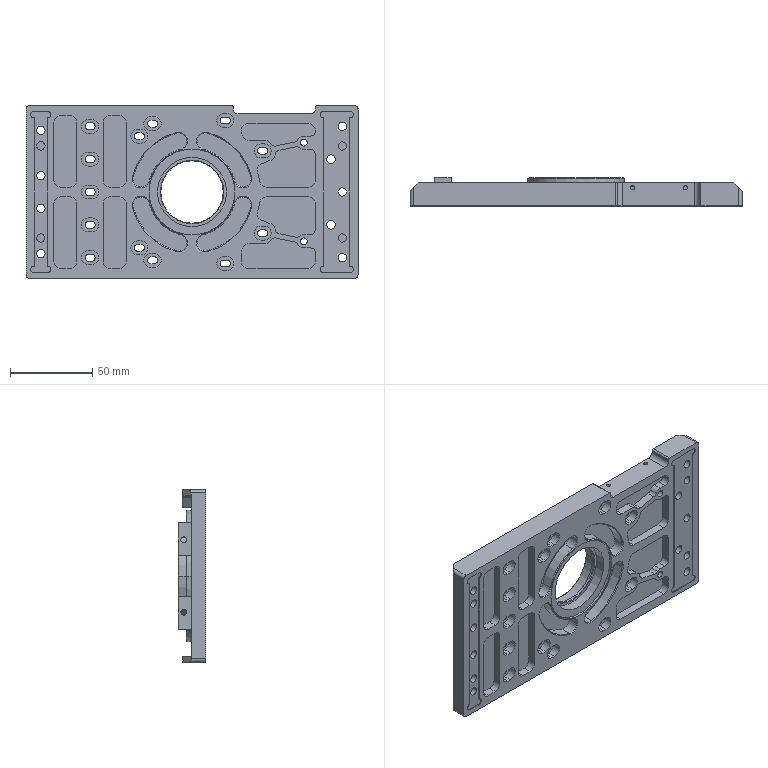Part | 1 solid | 393 faces | box 202 x 17 x 105 mm | volume 156849 mm3 | cylinder 196 | plane 171 | cone 26 | commonest cylinder face diameters 8 x36 4.2 x30 8.5 x26 5.2 x20 4 x17 6 x14